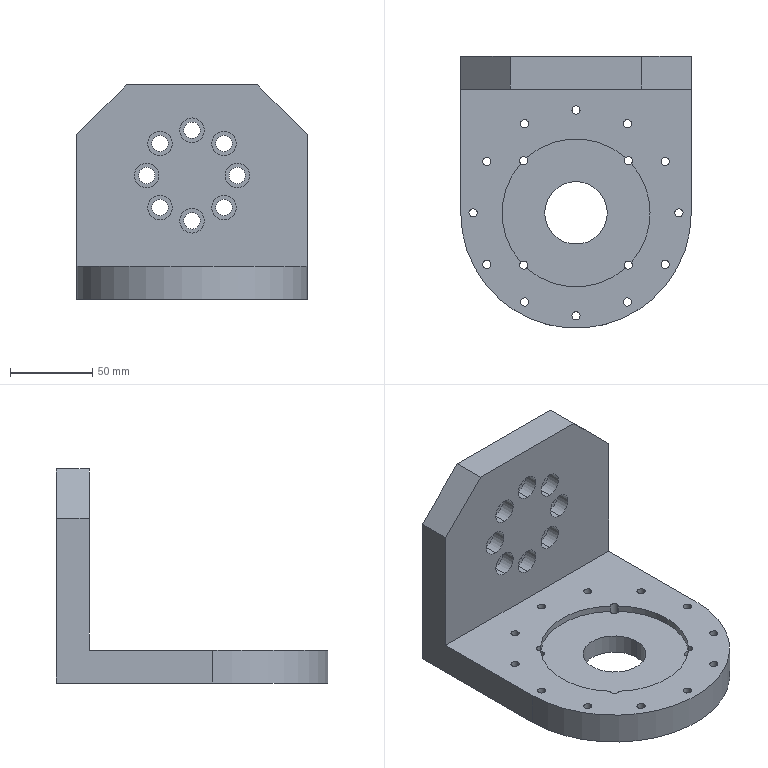Part | SolidWorks | features HoleWzd 5, ICE 4, Chamfer 1, Extrusion 1 | 1 solid | 107 faces | box 140 x 165 x 130 mm | volume 629581 mm3 | cylinder 79 | plane 23 | cone 5 | commonest cylinder face diameters 5 x37 10 x16 15 x16 90 x5 38 x2 70 x2